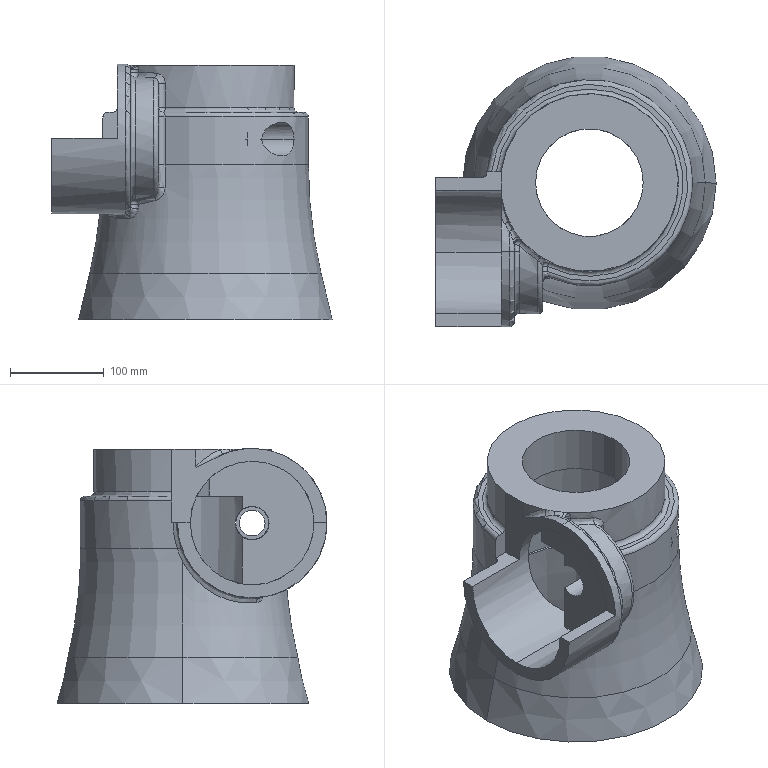Part | SolidWorks | features Cut 4, Fillet 4, ICE 4, Extrusion 1, Revolution 1 | 2 solids | 83 faces | box 299.386 x 289.264 x 272.746 mm | volume 5989690 mm3 | cylinder 30 | plane 21 | spline 15 | torus 9 | sphere 4 | cone 4 | commonest cylinder face diameters 10 x4 36 x4 159.756 x4 132.144 x3 161.466 x3 27.455 x2